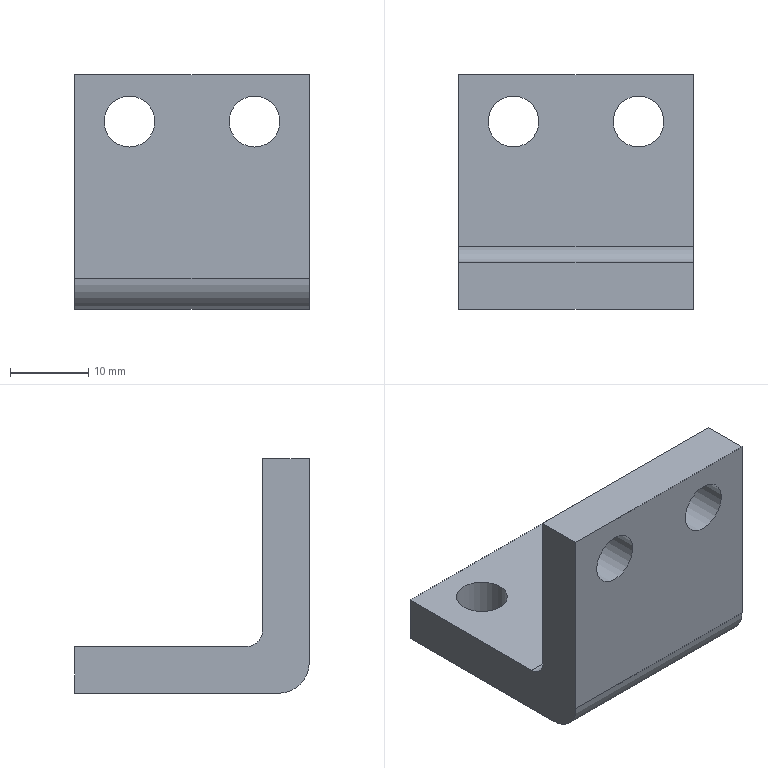Part | NX | features DATUM_CSYS 3, EXTRACT_BODY 2, SIMPLE HOLE 2, SKETCH 2, BLEND 1, Container 1, EXTRUDE 1, Geometry Instance 1, HOLE PACKAGE 1, SUBTRACT 1 | 1 solid | 14 faces | box 30 x 30 x 30 mm | volume 8846 mm3 | plane 8 | cylinder 6 | commonest cylinder face diameters 6.5 x4 4 x1 8 x1
STEP:
#1=CARTESIAN_POINT('',(-15.,4.,0.));
#2=VERTEX_POINT('',#1);
#3=CARTESIAN_POINT('',(-15.,30.,0.));
#4=VERTEX_POINT('',#3);
#5=CARTESIAN_POINT('',(-15.,4.,0.));
#6=DIRECTION('',(0.,1.,0.));
#7=VECTOR('',#6,1000.);
#8=LINE('',#5,#7);
#9=EDGE_CURVE('',#2,#4,#8,.T.);
#10=ORIENTED_EDGE('',*,*,#9,.F.);
#11=CARTESIAN_POINT('',(-15.,0.,4.));
#12=VERTEX_POINT('',#11);
#13=CARTESIAN_POINT('',(-15.,4.,4.));
#14=DIRECTION('',(1.,0.,0.));
#15=DIRECTION('',(0.,1.,0.));
#16=AXIS2_PLACEMENT_3D('',#13,#14,#15);
#17=CIRCLE('',#16,4.);
#18=EDGE_CURVE('',#12,#2,#17,.T.);
#19=ORIENTED_EDGE('',*,*,#18,.F.);
#20=CARTESIAN_POINT('',(-15.,0.,30.));
#21=VERTEX_POINT('',#20);
#22=CARTESIAN_POINT('',(-15.,0.,30.));
#23=DIRECTION('',(0.,0.,-1.));
#24=VECTOR('',#23,1000.);
#25=LINE('',#22,#24);
#26=EDGE_CURVE('',#21,#12,#25,.T.);
#27=ORIENTED_EDGE('',*,*,#26,.F.);
#28=CARTESIAN_POINT('',(-15.,6.,30.));
#29=VERTEX_POINT('',#28);
#30=CARTESIAN_POINT('',(-15.,0.,30.));
#31=DIRECTION('',(0.,-1.,0.));
#32=VECTOR('',#31,1000.);
#33=LINE('',#30,#32);
#34=EDGE_CURVE('',#21,#29,#33,.F.);
#35=ORIENTED_EDGE('',*,*,#34,.T.);
#36=CARTESIAN_POINT('',(-15.,6.,8.));
#37=VERTEX_POINT('',#36);
#38=CARTESIAN_POINT('',(-15.,6.,30.));
#39=DIRECTION('',(0.,0.,-1.));
#40=VECTOR('',#39,1000.);
#41=LINE('',#38,#40);
#42=EDGE_CURVE('',#29,#37,#41,.T.);
#43=ORIENTED_EDGE('',*,*,#42,.T.);
#44=CARTESIAN_POINT('',(-15.,8.,6.));
#45=VERTEX_POINT('',#44);
#46=CARTESIAN_POINT('',(-15.,8.,8.));
#47=DIRECTION('',(-1.,0.,0.));
#48=DIRECTION('',(0.,0.,1.));
#49=AXIS2_PLACEMENT_3D('',#46,#47,#48);
#50=CIRCLE('',#49,2.);
#51=EDGE_CURVE('',#37,#45,#50,.F.);
#52=ORIENTED_EDGE('',*,*,#51,.T.);
#53=CARTESIAN_POINT('',(-15.,30.,6.));
#54=VERTEX_POINT('',#53);
#55=CARTESIAN_POINT('',(-15.,4.,6.));
#56=DIRECTION('',(0.,1.,0.));
#57=VECTOR('',#56,1000.);
#58=LINE('',#55,#57);
#59=EDGE_CURVE('',#45,#54,#58,.T.);
#60=ORIENTED_EDGE('',*,*,#59,.T.);
#61=CARTESIAN_POINT('',(-15.,30.,0.));
#62=DIRECTION('',(0.,0.,-1.));
#63=VECTOR('',#62,1000.);
#64=LINE('',#61,#63);
#65=EDGE_CURVE('',#4,#54,#64,.F.);
#66=ORIENTED_EDGE('',*,*,#65,.F.);
#67=EDGE_LOOP('',(#10,#19,#27,#35,#43,#52,#60,#66));
#68=FACE_BOUND('',#67,.T.);
#69=CARTESIAN_POINT('',(-15.,4.,0.));
#70=DIRECTION('',(-1.,0.,0.));
#71=DIRECTION('',(0.,1.,0.));
#72=AXIS2_PLACEMENT_3D('',#69,#70,#71);
#73=PLANE('',#72);
#74=ADVANCED_FACE('',(#68),#73,.T.);
#75=ORIENTED_EDGE('',*,*,#65,.T.);
#76=CARTESIAN_POINT('',(15.,30.,6.));
#77=VERTEX_POINT('',#76);
#78=CARTESIAN_POINT('',(-15.,30.,6.));
#79=DIRECTION('',(-1.,0.,0.));
#80=VECTOR('',#79,1000.);
#81=LINE('',#78,#80);
#82=EDGE_CURVE('',#54,#77,#81,.F.);
#83=ORIENTED_EDGE('',*,*,#82,.T.);
#84=CARTESIAN_POINT('',(15.,30.,0.));
#85=VERTEX_POINT('',#84);
#86=CARTESIAN_POINT('',(15.,30.,0.));
#87=DIRECTION('',(0.,0.,-1.));
#88=VECTOR('',#87,1000.);
#89=LINE('',#86,#88);
#90=EDGE_CURVE('',#85,#77,#89,.F.);
#91=ORIENTED_EDGE('',*,*,#90,.F.);
#92=CARTESIAN_POINT('',(-15.,30.,0.));
#93=DIRECTION('',(1.,0.,0.));
#94=VECTOR('',#93,1000.);
#95=LINE('',#92,#94);
#96=EDGE_CURVE('',#4,#85,#95,.T.);
#97=ORIENTED_EDGE('',*,*,#96,.F.);
#98=EDGE_LOOP('',(#75,#83,#91,#97));
#99=FACE_BOUND('',#98,.T.);
#100=CARTESIAN_POINT('',(-15.,30.,0.));
#101=DIRECTION('',(0.,1.,0.));
#102=DIRECTION('',(1.,0.,0.));
#103=AXIS2_PLACEMENT_3D('',#100,#101,#102);
#104=PLANE('',#103);
#105=ADVANCED_FACE('',(#99),#104,.T.);
#106=CARTESIAN_POINT('',(15.,0.,30.));
#107=VERTEX_POINT('',#106);
#108=CARTESIAN_POINT('',(15.,0.,4.));
#109=VERTEX_POINT('',#108);
#110=CARTESIAN_POINT('',(15.,0.,30.));
#111=DIRECTION('',(0.,0.,-1.));
#112=VECTOR('',#111,1000.);
#113=LINE('',#110,#112);
#114=EDGE_CURVE('',#107,#109,#113,.T.);
#115=ORIENTED_EDGE('',*,*,#114,.T.);
#116=CARTESIAN_POINT('',(15.,4.,0.));
#117=VERTEX_POINT('',#116);
#118=CARTESIAN_POINT('',(15.,4.,4.));
#119=DIRECTION('',(1.,0.,0.));
#120=DIRECTION('',(0.,1.,0.));
#121=AXIS2_PLACEMENT_3D('',#118,#119,#120);
#122=CIRCLE('',#121,4.);
#123=EDGE_CURVE('',#109,#117,#122,.T.);
#124=ORIENTED_EDGE('',*,*,#123,.T.);
#125=CARTESIAN_POINT('',(15.,4.,0.));
#126=DIRECTION('',(0.,1.,0.));
#127=VECTOR('',#126,1000.);
#128=LINE('',#125,#127);
#129=EDGE_CURVE('',#117,#85,#128,.T.);
#130=ORIENTED_EDGE('',*,*,#129,.T.);
#131=ORIENTED_EDGE('',*,*,#90,.T.);
#132=CARTESIAN_POINT('',(15.,8.,6.));
#133=VERTEX_POINT('',#132);
#134=CARTESIAN_POINT('',(15.,4.,6.));
#135=DIRECTION('',(0.,1.,0.));
#136=VECTOR('',#135,1000.);
#137=LINE('',#134,#136);
#138=EDGE_CURVE('',#133,#77,#137,.T.);
#139=ORIENTED_EDGE('',*,*,#138,.F.);
#140=CARTESIAN_POINT('',(15.,6.,8.));
#141=VERTEX_POINT('',#140);
#142=CARTESIAN_POINT('',(15.,8.,8.));
#143=DIRECTION('',(-1.,0.,0.));
#144=DIRECTION('',(0.,0.,1.));
#145=AXIS2_PLACEMENT_3D('',#142,#143,#144);
#146=CIRCLE('',#145,2.);
#147=EDGE_CURVE('',#133,#141,#146,.T.);
#148=ORIENTED_EDGE('',*,*,#147,.T.);
#149=CARTESIAN_POINT('',(15.,6.,30.));
#150=VERTEX_POINT('',#149);
#151=CARTESIAN_POINT('',(15.,6.,30.));
#152=DIRECTION('',(0.,0.,-1.));
#153=VECTOR('',#152,1000.);
#154=LINE('',#151,#153);
#155=EDGE_CURVE('',#150,#141,#154,.T.);
#156=ORIENTED_EDGE('',*,*,#155,.F.);
#157=CARTESIAN_POINT('',(15.,0.,30.));
#158=DIRECTION('',(0.,-1.,0.));
#159=VECTOR('',#158,1000.);
#160=LINE('',#157,#159);
#161=EDGE_CURVE('',#107,#150,#160,.F.);
#162=ORIENTED_EDGE('',*,*,#161,.F.);
#163=EDGE_LOOP('',(#115,#124,#130,#131,#139,#148,#156,#162));
#164=FACE_BOUND('',#163,.T.);
#165=CARTESIAN_POINT('',(15.,0.,30.));
#166=DIRECTION('',(-1.,0.,0.));
#167=DIRECTION('',(0.,0.,-1.));
#168=AXIS2_PLACEMENT_3D('',#165,#166,#167);
#169=PLANE('',#168);
#170=ADVANCED_FACE('',(#164),#169,.F.);
#171=CARTESIAN_POINT('',(-15.,0.,30.));
#172=DIRECTION('',(1.,0.,0.));
#173=VECTOR('',#172,1000.);
#174=LINE('',#171,#173);
#175=EDGE_CURVE('',#21,#107,#174,.T.);
#176=ORIENTED_EDGE('',*,*,#175,.T.);
#177=ORIENTED_EDGE('',*,*,#161,.T.);
#178=CARTESIAN_POINT('',(-15.,6.,30.));
#179=DIRECTION('',(1.,0.,0.));
#180=VECTOR('',#179,1000.);
#181=LINE('',#178,#180);
#182=EDGE_CURVE('',#29,#150,#181,.T.);
#183=ORIENTED_EDGE('',*,*,#182,.F.);
#184=ORIENTED_EDGE('',*,*,#34,.F.);
#185=EDGE_LOOP('',(#176,#177,#183,#184));
#186=FACE_BOUND('',#185,.T.);
#187=CARTESIAN_POINT('',(-15.,0.,30.));
#188=DIRECTION('',(0.,0.,-1.));
#189=DIRECTION('',(1.,0.,0.));
#190=AXIS2_PLACEMENT_3D('',#187,#188,#189);
#191=PLANE('',#190);
#192=ADVANCED_FACE('',(#186),#191,.F.);
#193=CARTESIAN_POINT('',(8.,6.,20.75));
#194=VERTEX_POINT('',#193);
#195=CARTESIAN_POINT('',(8.,6.,24.));
#196=DIRECTION('',(0.,-1.,0.));
#197=DIRECTION('',(0.,0.,-1.));
#198=AXIS2_PLACEMENT_3D('',#195,#196,#197);
#199=CIRCLE('',#198,3.25);
#200=EDGE_CURVE('',#194,#194,#199,.T.);
#201=ORIENTED_EDGE('',*,*,#200,.T.);
#202=EDGE_LOOP('',(#201));
#203=FACE_BOUND('',#202,.T.);
#204=CARTESIAN_POINT('',(-8.,6.,20.75));
#205=VERTEX_POINT('',#204);
#206=CARTESIAN_POINT('',(-8.,6.,24.));
#207=DIRECTION('',(0.,-1.,0.));
#208=DIRECTION('',(0.,0.,-1.));
#209=AXIS2_PLACEMENT_3D('',#206,#207,#208);
#210=CIRCLE('',#209,3.25);
#211=EDGE_CURVE('',#205,#205,#210,.T.);
#212=ORIENTED_EDGE('',*,*,#211,.T.);
#213=EDGE_LOOP('',(#212));
#214=FACE_BOUND('',#213,.T.);
#215=ORIENTED_EDGE('',*,*,#155,.T.);
#216=CARTESIAN_POINT('',(-15.,6.,8.));
#217=DIRECTION('',(1.,0.,0.));
#218=VECTOR('',#217,1000.);
#219=LINE('',#216,#218);
#220=EDGE_CURVE('',#141,#37,#219,.F.);
#221=ORIENTED_EDGE('',*,*,#220,.T.);
#222=ORIENTED_EDGE('',*,*,#42,.F.);
#223=ORIENTED_EDGE('',*,*,#182,.T.);
#224=EDGE_LOOP('',(#215,#221,#222,#223));
#225=FACE_BOUND('',#224,.T.);
#226=CARTESIAN_POINT('',(-15.,6.,30.));
#227=DIRECTION('',(0.,-1.,0.));
#228=DIRECTION('',(0.,0.,-1.));
#229=AXIS2_PLACEMENT_3D('',#226,#227,#228);
#230=PLANE('',#229);
#231=ADVANCED_FACE('',(#203,#214,#225),#230,.F.);
#232=CARTESIAN_POINT('',(-8.,20.75,6.));
#233=VERTEX_POINT('',#232);
#234=CARTESIAN_POINT('',(-8.,24.,6.));
#235=DIRECTION('',(0.,0.,1.));
#236=DIRECTION('',(0.,-1.,0.));
#237=AXIS2_PLACEMENT_3D('',#234,#235,#236);
#238=CIRCLE('',#237,3.25);
#239=EDGE_CURVE('',#233,#233,#238,.F.);
#240=ORIENTED_EDGE('',*,*,#239,.T.);
#241=EDGE_LOOP('',(#240));
#242=FACE_BOUND('',#241,.T.);
#243=CARTESIAN_POINT('',(8.,20.75,6.));
#244=VERTEX_POINT('',#243);
#245=CARTESIAN_POINT('',(8.,24.,6.));
#246=DIRECTION('',(0.,0.,1.));
#247=DIRECTION('',(0.,-1.,0.));
#248=AXIS2_PLACEMENT_3D('',#245,#246,#247);
#249=CIRCLE('',#248,3.25);
#250=EDGE_CURVE('',#244,#244,#249,.F.);
#251=ORIENTED_EDGE('',*,*,#250,.T.);
#252=EDGE_LOOP('',(#251));
#253=FACE_BOUND('',#252,.T.);
#254=ORIENTED_EDGE('',*,*,#59,.F.);
#255=CARTESIAN_POINT('',(15.,8.,6.));
#256=DIRECTION('',(1.,0.,0.));
#257=VECTOR('',#256,1000.);
#258=LINE('',#255,#257);
#259=EDGE_CURVE('',#45,#133,#258,.T.);
#260=ORIENTED_EDGE('',*,*,#259,.T.);
#261=ORIENTED_EDGE('',*,*,#138,.T.);
#262=ORIENTED_EDGE('',*,*,#82,.F.);
#263=EDGE_LOOP('',(#254,#260,#261,#262));
#264=FACE_BOUND('',#263,.T.);
#265=CARTESIAN_POINT('',(-15.,4.,6.));
#266=DIRECTION('',(0.,0.,-1.));
#267=DIRECTION('',(-1.,0.,0.));
#268=AXIS2_PLACEMENT_3D('',#265,#266,#267);
#269=PLANE('',#268);
#270=ADVANCED_FACE('',(#242,#253,#264),#269,.F.);
#271=CARTESIAN_POINT('',(8.,0.,20.75));
#272=VERTEX_POINT('',#271);
#273=CARTESIAN_POINT('',(8.,0.,24.));
#274=DIRECTION('',(0.,-1.,0.));
#275=DIRECTION('',(0.,0.,-1.));
#276=AXIS2_PLACEMENT_3D('',#273,#274,#275);
#277=CIRCLE('',#276,3.25);
#278=EDGE_CURVE('',#272,#272,#277,.T.);
#279=ORIENTED_EDGE('',*,*,#278,.F.);
#280=EDGE_LOOP('',(#279));
#281=FACE_BOUND('',#280,.T.);
#282=CARTESIAN_POINT('',(-8.,0.,20.75));
#283=VERTEX_POINT('',#282);
#284=CARTESIAN_POINT('',(-8.,0.,24.));
#285=DIRECTION('',(0.,-1.,0.));
#286=DIRECTION('',(0.,0.,-1.));
#287=AXIS2_PLACEMENT_3D('',#284,#285,#286);
#288=CIRCLE('',#287,3.25);
#289=EDGE_CURVE('',#283,#283,#288,.T.);
#290=ORIENTED_EDGE('',*,*,#289,.F.);
#291=EDGE_LOOP('',(#290));
#292=FACE_BOUND('',#291,.T.);
#293=ORIENTED_EDGE('',*,*,#114,.F.);
#294=ORIENTED_EDGE('',*,*,#175,.F.);
#295=ORIENTED_EDGE('',*,*,#26,.T.);
#296=CARTESIAN_POINT('',(-15.,0.,4.));
#297=DIRECTION('',(1.,0.,0.));
#298=VECTOR('',#297,1000.);
#299=LINE('',#296,#298);
#300=EDGE_CURVE('',#12,#109,#299,.T.);
#301=ORIENTED_EDGE('',*,*,#300,.T.);
#302=EDGE_LOOP('',(#293,#294,#295,#301));
#303=FACE_BOUND('',#302,.T.);
#304=CARTESIAN_POINT('',(-15.,0.,30.));
#305=DIRECTION('',(0.,-1.,0.));
#306=DIRECTION('',(0.,0.,-1.));
#307=AXIS2_PLACEMENT_3D('',#304,#305,#306);
#308=PLANE('',#307);
#309=ADVANCED_FACE('',(#281,#292,#303),#308,.T.);
#310=ORIENTED_EDGE('',*,*,#123,.F.);
#311=ORIENTED_EDGE('',*,*,#300,.F.);
#312=ORIENTED_EDGE('',*,*,#18,.T.);
#313=CARTESIAN_POINT('',(-15.,4.,0.));
#314=DIRECTION('',(1.,0.,0.));
#315=VECTOR('',#314,1000.);
#316=LINE('',#313,#315);
#317=EDGE_CURVE('',#2,#117,#316,.T.);
#318=ORIENTED_EDGE('',*,*,#317,.T.);
#319=EDGE_LOOP('',(#310,#311,#312,#318));
#320=FACE_BOUND('',#319,.T.);
#321=CARTESIAN_POINT('',(-15.,4.,4.));
#322=DIRECTION('',(1.,0.,0.));
#323=DIRECTION('',(0.,0.,-1.));
#324=AXIS2_PLACEMENT_3D('',#321,#322,#323);
#325=CYLINDRICAL_SURFACE('',#324,4.);
#326=ADVANCED_FACE('',(#320),#325,.T.);
#327=CARTESIAN_POINT('',(-8.,20.75,0.));
#328=VERTEX_POINT('',#327);
#329=CARTESIAN_POINT('',(-8.,24.,0.));
#330=DIRECTION('',(0.,0.,1.));
#331=DIRECTION('',(0.,-1.,0.));
#332=AXIS2_PLACEMENT_3D('',#329,#330,#331);
#333=CIRCLE('',#332,3.25);
#334=EDGE_CURVE('',#328,#328,#333,.F.);
#335=ORIENTED_EDGE('',*,*,#334,.F.);
#336=EDGE_LOOP('',(#335));
#337=FACE_BOUND('',#336,.T.);
#338=CARTESIAN_POINT('',(8.,20.75,0.));
#339=VERTEX_POINT('',#338);
#340=CARTESIAN_POINT('',(8.,24.,0.));
#341=DIRECTION('',(0.,0.,1.));
#342=DIRECTION('',(0.,-1.,0.));
#343=AXIS2_PLACEMENT_3D('',#340,#341,#342);
#344=CIRCLE('',#343,3.25);
#345=EDGE_CURVE('',#339,#339,#344,.F.);
#346=ORIENTED_EDGE('',*,*,#345,.F.);
#347=EDGE_LOOP('',(#346));
#348=FACE_BOUND('',#347,.T.);
#349=ORIENTED_EDGE('',*,*,#129,.F.);
#350=ORIENTED_EDGE('',*,*,#317,.F.);
#351=ORIENTED_EDGE('',*,*,#9,.T.);
#352=ORIENTED_EDGE('',*,*,#96,.T.);
#353=EDGE_LOOP('',(#349,#350,#351,#352));
#354=FACE_BOUND('',#353,.T.);
#355=CARTESIAN_POINT('',(-15.,4.,0.));
#356=DIRECTION('',(0.,0.,-1.));
#357=DIRECTION('',(-1.,0.,0.));
#358=AXIS2_PLACEMENT_3D('',#355,#356,#357);
#359=PLANE('',#358);
#360=ADVANCED_FACE('',(#337,#348,#354),#359,.T.);
#361=ORIENTED_EDGE('',*,*,#51,.F.);
#362=ORIENTED_EDGE('',*,*,#220,.F.);
#363=ORIENTED_EDGE('',*,*,#147,.F.);
#364=ORIENTED_EDGE('',*,*,#259,.F.);
#365=EDGE_LOOP('',(#361,#362,#363,#364));
#366=FACE_BOUND('',#365,.T.);
#367=CARTESIAN_POINT('',(-15.,8.,8.));
#368=DIRECTION('',(-1.,0.,0.));
#369=DIRECTION('',(0.,0.,1.));
#370=AXIS2_PLACEMENT_3D('',#367,#368,#369);
#371=CYLINDRICAL_SURFACE('',#370,2.);
#372=ADVANCED_FACE('',(#366),#371,.F.);
#373=ORIENTED_EDGE('',*,*,#289,.T.);
#374=EDGE_LOOP('',(#373));
#375=FACE_BOUND('',#374,.T.);
#376=ORIENTED_EDGE('',*,*,#211,.F.);
#377=EDGE_LOOP('',(#376));
#378=FACE_BOUND('',#377,.T.);
#379=CARTESIAN_POINT('',(-8.,6.,24.));
#380=DIRECTION('',(0.,-1.,0.));
#381=DIRECTION('',(0.,0.,-1.));
#382=AXIS2_PLACEMENT_3D('',#379,#380,#381);
#383=CYLINDRICAL_SURFACE('',#382,3.25);
#384=ADVANCED_FACE('',(#375,#378),#383,.F.);
#385=ORIENTED_EDGE('',*,*,#278,.T.);
#386=EDGE_LOOP('',(#385));
#387=FACE_BOUND('',#386,.T.);
#388=ORIENTED_EDGE('',*,*,#200,.F.);
#389=EDGE_LOOP('',(#388));
#390=FACE_BOUND('',#389,.T.);
#391=CARTESIAN_POINT('',(8.,6.,24.));
#392=DIRECTION('',(0.,-1.,0.));
#393=DIRECTION('',(0.,0.,-1.));
#394=AXIS2_PLACEMENT_3D('',#391,#392,#393);
#395=CYLINDRICAL_SURFACE('',#394,3.25);
#396=ADVANCED_FACE('',(#387,#390),#395,.F.);
#397=ORIENTED_EDGE('',*,*,#345,.T.);
#398=EDGE_LOOP('',(#397));
#399=FACE_BOUND('',#398,.T.);
#400=ORIENTED_EDGE('',*,*,#250,.F.);
#401=EDGE_LOOP('',(#400));
#402=FACE_BOUND('',#401,.T.);
#403=CARTESIAN_POINT('',(8.,24.,6.));
#404=DIRECTION('',(0.,0.,-1.));
#405=DIRECTION('',(0.,-1.,0.));
#406=AXIS2_PLACEMENT_3D('',#403,#404,#405);
#407=CYLINDRICAL_SURFACE('',#406,3.25);
#408=ADVANCED_FACE('',(#399,#402),#407,.F.);
#409=ORIENTED_EDGE('',*,*,#334,.T.);
#410=EDGE_LOOP('',(#409));
#411=FACE_BOUND('',#410,.T.);
#412=ORIENTED_EDGE('',*,*,#239,.F.);
#413=EDGE_LOOP('',(#412));
#414=FACE_BOUND('',#413,.T.);
#415=CARTESIAN_POINT('',(-8.,24.,6.));
#416=DIRECTION('',(0.,0.,-1.));
#417=DIRECTION('',(0.,-1.,0.));
#418=AXIS2_PLACEMENT_3D('',#415,#416,#417);
#419=CYLINDRICAL_SURFACE('',#418,3.25);
#420=ADVANCED_FACE('',(#411,#414),#419,.F.);
#421=CLOSED_SHELL('',(#74,#105,#170,#192,#231,#270,#309,#326,#360,#372,#384,#396,#408,#420));
#422=MANIFOLD_SOLID_BREP('',#421);
#423=(LENGTH_UNIT()NAMED_UNIT(*)SI_UNIT(.MILLI.,.METRE.));
#424=UNCERTAINTY_MEASURE_WITH_UNIT(LENGTH_MEASURE(0.00001),#423,'','');
#425=(NAMED_UNIT(*)PLANE_ANGLE_UNIT()SI_UNIT($,.RADIAN.));
#426=(NAMED_UNIT(*)SI_UNIT($,.STERADIAN.)SOLID_ANGLE_UNIT());
#427=(GEOMETRIC_REPRESENTATION_CONTEXT(3)GLOBAL_UNCERTAINTY_ASSIGNED_CONTEXT((#424))GLOBAL_UNIT_ASSIGNED_CONTEXT((#423,#425,#426))REPRESENTATION_CONTEXT('',''));
#428=ADVANCED_BREP_SHAPE_REPRESENTATION('',(#422),#427);